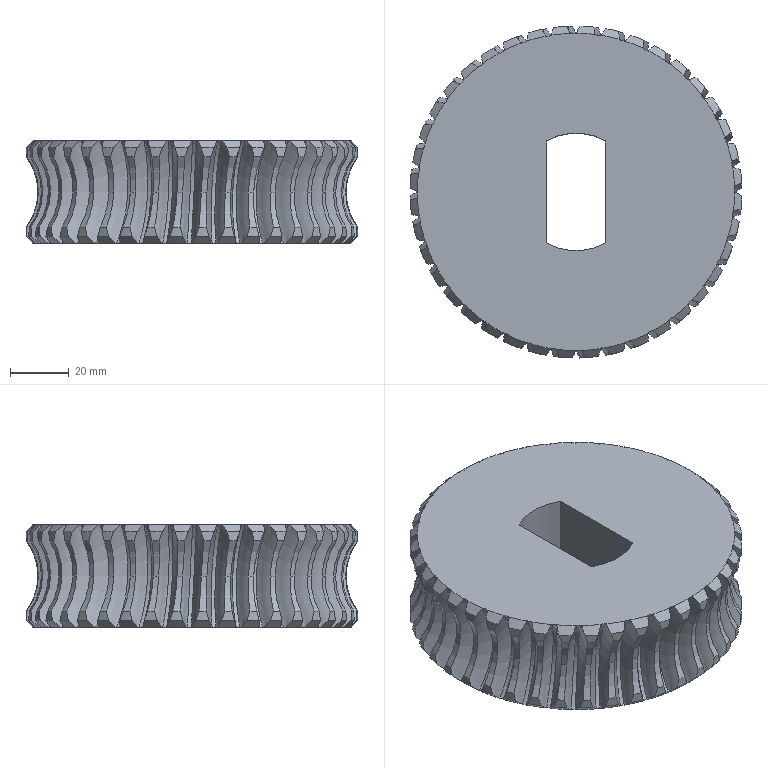Part | SolidWorks | 1 solid | 368 faces | box 112.877 x 112.877 x 35 mm | volume 271354 mm3 | spline 120 | cone 82 | cylinder 82 | torus 80 | plane 4 | commonest cylinder face diameters 112.906 x80 40 x2